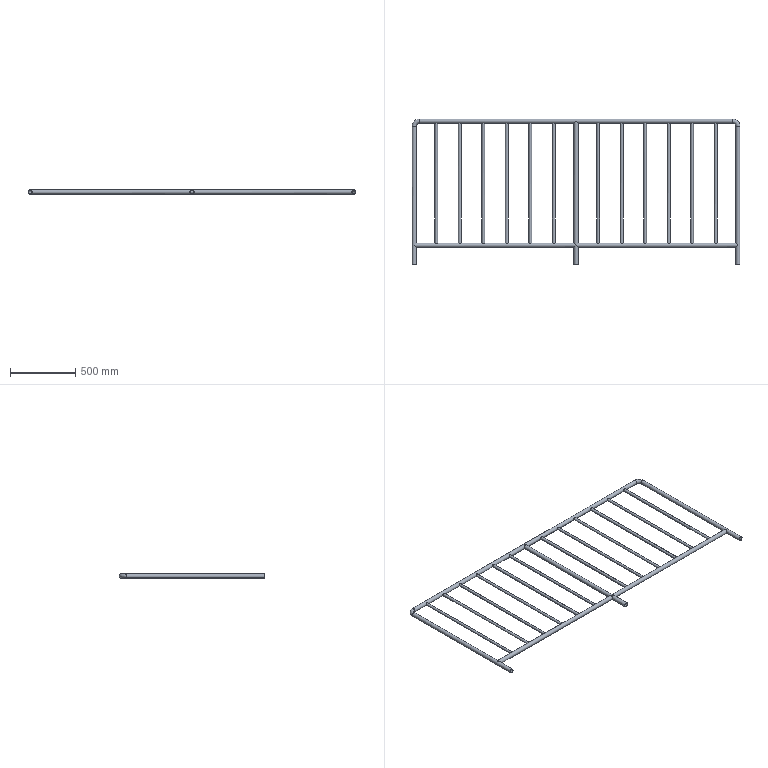Part | STEP file | PN_0004 304 guardrail 2480X1100 body_Default<As Machined> | 20 solids | 80 faces | box 2512 x 1116 x 32 mm | volume 1834535 mm3 | cylinder 65 | plane 11 | torus 4 | commonest cylinder face diameters 32 x35 18 x12 20 x12 29 x6